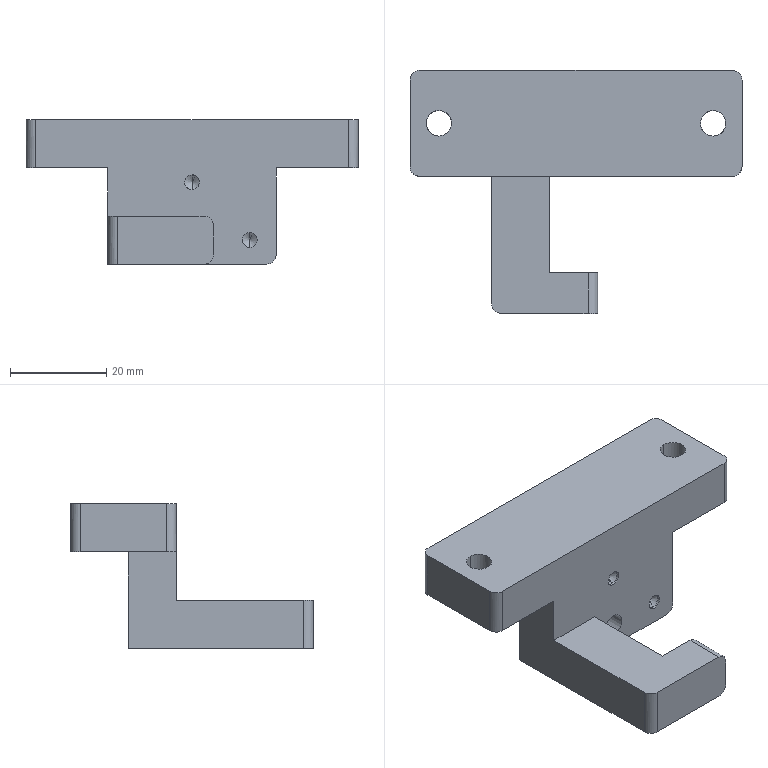Part | 1 solid | 49 faces | box 69 x 50.5 x 30 mm | volume 25530 mm3 | cylinder 24 | plane 15 | cone 10 | commonest cylinder face diameters 4 x8 2.5 x4 3.1 x4 5 x4 5.3 x4